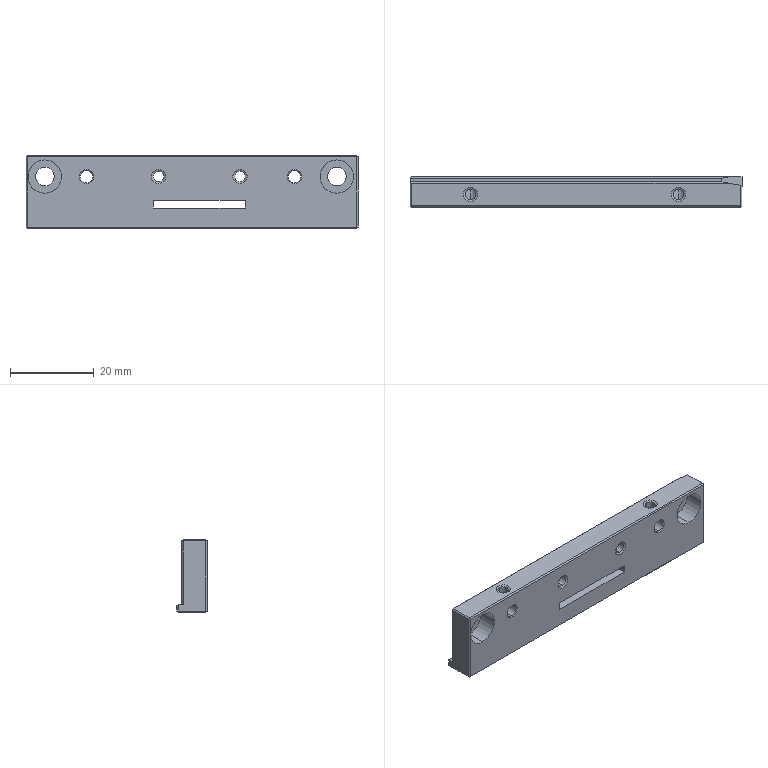Part | NX | 1 solid | 61 faces | box 79.5 x 7.2 x 17.4 mm | volume 7490 mm3 | plane 29 | cylinder 20 | cone 12 | commonest cylinder face diameters 2.5 x8 3 x4 4.5 x4 8 x4